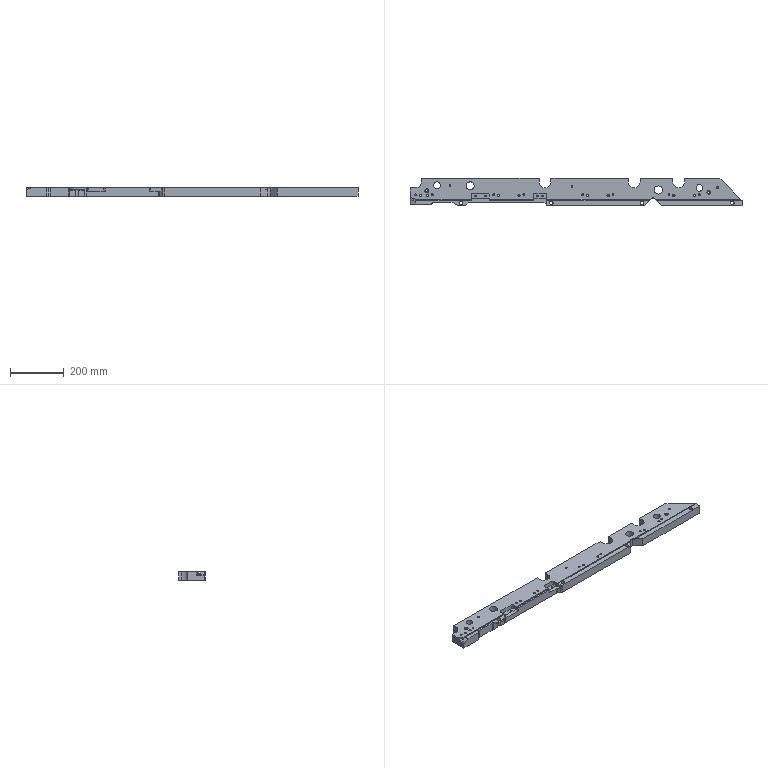Part | STEP file | gslz 2016.10.28-13_id322_x_t | 1 solid | 170 faces | box 1230 x 100 x 32 mm | volume 3247555 mm3 | cylinder 79 | plane 70 | cone 21 | commonest cylinder face diameters 6.8 x19 10 x14 6 x10 8 x8 18 x7 5.2 x4